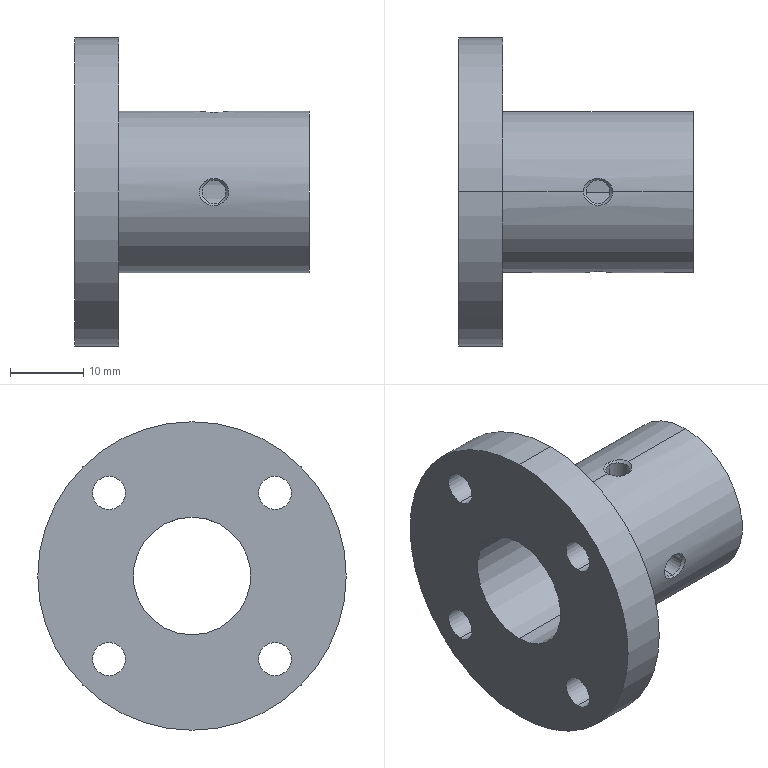Part | STEP file | STHRB16_STHRB16 | 1 solid | 35 faces | box 32 x 42 x 42 mm | volume 11327 mm3 | cylinder 24 | cone 8 | plane 3 | commonest cylinder face diameters 4.5 x8 4 x6 3.242 x4 16 x2 22 x2 42 x2
STEP:
#1=CARTESIAN_POINT('',(19.,-1.621,10.621));
#2=VERTEX_POINT('',#1);
#3=CARTESIAN_POINT('',(19.,1.621,10.621));
#4=VERTEX_POINT('',#3);
#5=CARTESIAN_POINT('',(19.,0.,10.621));
#6=DIRECTION('',(0.,0.,-1.));
#7=DIRECTION('',(0.,1.,0.));
#8=AXIS2_PLACEMENT_3D('',#5,#6,#7);
#9=CIRCLE('',#8,1.621);
#10=EDGE_CURVE('',#2,#4,#9,.T.);
#11=ORIENTED_EDGE('',*,*,#10,.F.);
#12=CARTESIAN_POINT('',(19.,-1.621,8.379));
#13=VERTEX_POINT('',#12);
#14=CARTESIAN_POINT('',(19.,-1.621,11.));
#15=DIRECTION('',(0.,0.,-1.));
#16=VECTOR('',#15,1000.);
#17=LINE('',#14,#16);
#18=EDGE_CURVE('',#2,#13,#17,.T.);
#19=ORIENTED_EDGE('',*,*,#18,.T.);
#20=CARTESIAN_POINT('',(19.,1.621,8.379));
#21=VERTEX_POINT('',#20);
#22=CARTESIAN_POINT('',(19.,0.,8.379));
#23=DIRECTION('',(0.,0.,-1.));
#24=DIRECTION('',(0.,1.,0.));
#25=AXIS2_PLACEMENT_3D('',#22,#23,#24);
#26=CIRCLE('',#25,1.621);
#27=EDGE_CURVE('',#13,#21,#26,.T.);
#28=ORIENTED_EDGE('',*,*,#27,.T.);
#29=CARTESIAN_POINT('',(19.,1.621,11.));
#30=DIRECTION('',(0.,0.,-1.));
#31=VECTOR('',#30,1000.);
#32=LINE('',#29,#31);
#33=EDGE_CURVE('',#4,#21,#32,.T.);
#34=ORIENTED_EDGE('',*,*,#33,.F.);
#35=EDGE_LOOP('',(#11,#19,#28,#34));
#36=FACE_OUTER_BOUND('',#35,.T.);
#37=CARTESIAN_POINT('',(19.,0.,11.));
#38=DIRECTION('',(0.,0.,-1.));
#39=DIRECTION('',(0.,1.,0.));
#40=AXIS2_PLACEMENT_3D('',#37,#38,#39);
#41=CYLINDRICAL_SURFACE('',#40,1.621);
#42=ADVANCED_FACE('',(#36),#41,.F.);
#43=ORIENTED_EDGE('',*,*,#27,.F.);
#44=CARTESIAN_POINT('',(19.,-2.,8.));
#45=VERTEX_POINT('',#44);
#46=CARTESIAN_POINT('',(19.,-1.621,8.379));
#47=DIRECTION('',(0.,-0.7071,-0.7071));
#48=VECTOR('',#47,1000.);
#49=LINE('',#46,#48);
#50=EDGE_CURVE('',#13,#45,#49,.T.);
#51=ORIENTED_EDGE('',*,*,#50,.T.);
#52=CARTESIAN_POINT('',(17.,0.,8.));
#53=VERTEX_POINT('',#52);
#54=CARTESIAN_POINT('',(19.,0.,8.));
#55=DIRECTION('',(0.,0.,-1.));
#56=DIRECTION('',(0.,1.,0.));
#57=AXIS2_PLACEMENT_3D('',#54,#55,#56);
#58=CIRCLE('',#57,2.);
#59=EDGE_CURVE('',#45,#53,#58,.T.);
#60=ORIENTED_EDGE('',*,*,#59,.T.);
#61=CARTESIAN_POINT('',(19.,2.,8.));
#62=VERTEX_POINT('',#61);
#63=CARTESIAN_POINT('',(19.,0.,8.));
#64=DIRECTION('',(0.,0.,-1.));
#65=DIRECTION('',(0.,1.,0.));
#66=AXIS2_PLACEMENT_3D('',#63,#64,#65);
#67=CIRCLE('',#66,2.);
#68=EDGE_CURVE('',#53,#62,#67,.T.);
#69=ORIENTED_EDGE('',*,*,#68,.T.);
#70=CARTESIAN_POINT('',(19.,1.621,8.379));
#71=DIRECTION('',(0.,0.7071,-0.7071));
#72=VECTOR('',#71,1000.);
#73=LINE('',#70,#72);
#74=EDGE_CURVE('',#21,#62,#73,.T.);
#75=ORIENTED_EDGE('',*,*,#74,.F.);
#76=EDGE_LOOP('',(#43,#51,#60,#69,#75));
#77=FACE_OUTER_BOUND('',#76,.T.);
#78=CARTESIAN_POINT('',(19.,0.,8.379));
#79=DIRECTION('',(0.,0.,-1.));
#80=DIRECTION('',(0.,1.,0.));
#81=AXIS2_PLACEMENT_3D('',#78,#79,#80);
#82=CONICAL_SURFACE('',#81,1.621,0.7854);
#83=ADVANCED_FACE('',(#77),#82,.F.);
#84=ORIENTED_EDGE('',*,*,#10,.T.);
#85=CARTESIAN_POINT('',(19.,1.844,10.844));
#86=VERTEX_POINT('',#85);
#87=CARTESIAN_POINT('',(19.,2.,11.));
#88=DIRECTION('',(0.,0.7071,0.7071));
#89=VECTOR('',#88,1000.);
#90=LINE('',#87,#89);
#91=EDGE_CURVE('',#4,#86,#90,.T.);
#92=ORIENTED_EDGE('',*,*,#91,.T.);
#93=CARTESIAN_POINT('',(17.,0.,11.));
#94=VERTEX_POINT('',#93);
#95=CARTESIAN_POINT('',(19.,1.844,10.844));
#96=CARTESIAN_POINT('',(18.874,1.844,10.844));
#97=CARTESIAN_POINT('',(18.747,1.833,10.846));
#98=CARTESIAN_POINT('',(18.499,1.789,10.854));
#99=CARTESIAN_POINT('',(18.378,1.756,10.859));
#100=CARTESIAN_POINT('',(18.142,1.669,10.873));
#101=CARTESIAN_POINT('',(18.027,1.615,10.881));
#102=CARTESIAN_POINT('',(17.811,1.486,10.899));
#103=CARTESIAN_POINT('',(17.71,1.413,10.909));
#104=CARTESIAN_POINT('',(17.522,1.247,10.929));
#105=CARTESIAN_POINT('',(17.435,1.153,10.94));
#106=CARTESIAN_POINT('',(17.284,0.9535,10.959));
#107=CARTESIAN_POINT('',(17.219,0.8468,10.968));
#108=CARTESIAN_POINT('',(17.058,0.5039,10.991));
#109=CARTESIAN_POINT('',(17.,0.2536,11.));
#110=CARTESIAN_POINT('',(17.,0.,11.));
#111=B_SPLINE_CURVE_WITH_KNOTS('',3,(#95,#96,#97,#98,#99,#100,#101,#102,#103,#104,#105,#106,#107,#108,#109,#110),.UNSPECIFIED.,.F.,.F.,(4,2,2,2,2,2,2,4),(0.007522,0.0079,0.008277,0.008655,0.009033,0.009411,0.009788,0.01054),.UNSPECIFIED.);
#112=EDGE_CURVE('',#86,#94,#111,.T.);
#113=ORIENTED_EDGE('',*,*,#112,.T.);
#114=CARTESIAN_POINT('',(19.,-1.844,10.844));
#115=VERTEX_POINT('',#114);
#116=CARTESIAN_POINT('',(17.,0.,11.));
#117=CARTESIAN_POINT('',(17.,-0.1265,11.));
#118=CARTESIAN_POINT('',(17.014,-0.2511,10.998));
#119=CARTESIAN_POINT('',(17.069,-0.4966,10.989));
#120=CARTESIAN_POINT('',(17.111,-0.6176,10.983));
#121=CARTESIAN_POINT('',(17.271,-0.958,10.961));
#122=CARTESIAN_POINT('',(17.427,-1.163,10.94));
#123=CARTESIAN_POINT('',(17.711,-1.414,10.909));
#124=CARTESIAN_POINT('',(17.813,-1.488,10.899));
#125=CARTESIAN_POINT('',(18.029,-1.616,10.881));
#126=CARTESIAN_POINT('',(18.144,-1.67,10.873));
#127=CARTESIAN_POINT('',(18.379,-1.757,10.859));
#128=CARTESIAN_POINT('',(18.5,-1.789,10.854));
#129=CARTESIAN_POINT('',(18.748,-1.833,10.846));
#130=CARTESIAN_POINT('',(18.875,-1.844,10.844));
#131=CARTESIAN_POINT('',(19.,-1.844,10.844));
#132=B_SPLINE_CURVE_WITH_KNOTS('',3,(#116,#117,#118,#119,#120,#121,#122,#123,#124,#125,#126,#127,#128,#129,#130,#131),.UNSPECIFIED.,.F.,.F.,(4,2,2,2,2,2,2,4),(0.01054,0.01092,0.0113,0.01205,0.01243,0.01281,0.01318,0.01356),.UNSPECIFIED.);
#133=EDGE_CURVE('',#94,#115,#132,.T.);
#134=ORIENTED_EDGE('',*,*,#133,.T.);
#135=CARTESIAN_POINT('',(19.,-2.,11.));
#136=DIRECTION('',(0.,-0.7071,0.7071));
#137=VECTOR('',#136,1000.);
#138=LINE('',#135,#137);
#139=EDGE_CURVE('',#2,#115,#138,.T.);
#140=ORIENTED_EDGE('',*,*,#139,.F.);
#141=EDGE_LOOP('',(#84,#92,#113,#134,#140));
#142=FACE_OUTER_BOUND('',#141,.T.);
#143=CARTESIAN_POINT('',(19.,0.,11.));
#144=DIRECTION('',(0.,0.,1.));
#145=DIRECTION('',(0.,-1.,0.));
#146=AXIS2_PLACEMENT_3D('',#143,#144,#145);
#147=CONICAL_SURFACE('',#146,2.,0.7854);
#148=ADVANCED_FACE('',(#142),#147,.F.);
#149=CARTESIAN_POINT('',(21.,0.,8.));
#150=VERTEX_POINT('',#149);
#151=CARTESIAN_POINT('',(19.,0.,8.));
#152=DIRECTION('',(0.,0.,-1.));
#153=DIRECTION('',(0.,1.,0.));
#154=AXIS2_PLACEMENT_3D('',#151,#152,#153);
#155=CIRCLE('',#154,2.);
#156=EDGE_CURVE('',#62,#150,#155,.T.);
#157=ORIENTED_EDGE('',*,*,#156,.F.);
#158=CARTESIAN_POINT('',(19.,2.,7.746));
#159=VERTEX_POINT('',#158);
#160=CARTESIAN_POINT('',(19.,2.,11.));
#161=DIRECTION('',(0.,0.,-1.));
#162=VECTOR('',#161,1000.);
#163=LINE('',#160,#162);
#164=EDGE_CURVE('',#62,#159,#163,.T.);
#165=ORIENTED_EDGE('',*,*,#164,.T.);
#166=CARTESIAN_POINT('',(19.,2.,7.746));
#167=CARTESIAN_POINT('',(19.132,2.,7.746));
#168=CARTESIAN_POINT('',(19.262,1.987,7.749));
#169=CARTESIAN_POINT('',(19.519,1.936,7.762));
#170=CARTESIAN_POINT('',(19.646,1.897,7.772));
#171=CARTESIAN_POINT('',(20.008,1.747,7.808));
#172=CARTESIAN_POINT('',(20.23,1.598,7.841));
#173=CARTESIAN_POINT('',(20.597,1.231,7.907));
#174=CARTESIAN_POINT('',(20.746,1.009,7.94));
#175=CARTESIAN_POINT('',(20.896,0.6485,7.975));
#176=CARTESIAN_POINT('',(20.935,0.5211,7.984));
#177=CARTESIAN_POINT('',(20.987,0.2634,7.997));
#178=CARTESIAN_POINT('',(21.,0.1326,8.));
#179=CARTESIAN_POINT('',(21.,0.,8.));
#180=B_SPLINE_CURVE_WITH_KNOTS('',3,(#166,#167,#168,#169,#170,#171,#172,#173,#174,#175,#176,#177,#178,#179),.UNSPECIFIED.,.F.,.F.,(4,2,2,2,2,2,4),(0.009417,0.009809,0.0102,0.01099,0.01177,0.01216,0.01255),.UNSPECIFIED.);
#181=EDGE_CURVE('',#159,#150,#180,.T.);
#182=ORIENTED_EDGE('',*,*,#181,.T.);
#183=EDGE_LOOP('',(#157,#165,#182));
#184=FACE_OUTER_BOUND('',#183,.T.);
#185=CARTESIAN_POINT('',(19.,0.,11.));
#186=DIRECTION('',(0.,0.,-1.));
#187=DIRECTION('',(0.,1.,0.));
#188=AXIS2_PLACEMENT_3D('',#185,#186,#187);
#189=CYLINDRICAL_SURFACE('',#188,2.);
#190=ADVANCED_FACE('',(#184),#189,.F.);
#191=CARTESIAN_POINT('',(19.,-10.621,-1.621));
#192=VERTEX_POINT('',#191);
#193=CARTESIAN_POINT('',(19.,-10.621,1.621));
#194=VERTEX_POINT('',#193);
#195=CARTESIAN_POINT('',(19.,-10.621,0.));
#196=DIRECTION('',(0.,1.,0.));
#197=DIRECTION('',(0.,0.,1.));
#198=AXIS2_PLACEMENT_3D('',#195,#196,#197);
#199=CIRCLE('',#198,1.621);
#200=EDGE_CURVE('',#192,#194,#199,.T.);
#201=ORIENTED_EDGE('',*,*,#200,.F.);
#202=CARTESIAN_POINT('',(19.,-8.379,-1.621));
#203=VERTEX_POINT('',#202);
#204=CARTESIAN_POINT('',(19.,-11.,-1.621));
#205=DIRECTION('',(0.,1.,0.));
#206=VECTOR('',#205,1000.);
#207=LINE('',#204,#206);
#208=EDGE_CURVE('',#192,#203,#207,.T.);
#209=ORIENTED_EDGE('',*,*,#208,.T.);
#210=CARTESIAN_POINT('',(19.,-8.379,1.621));
#211=VERTEX_POINT('',#210);
#212=CARTESIAN_POINT('',(19.,-8.379,0.));
#213=DIRECTION('',(0.,1.,0.));
#214=DIRECTION('',(0.,0.,1.));
#215=AXIS2_PLACEMENT_3D('',#212,#213,#214);
#216=CIRCLE('',#215,1.621);
#217=EDGE_CURVE('',#203,#211,#216,.T.);
#218=ORIENTED_EDGE('',*,*,#217,.T.);
#219=CARTESIAN_POINT('',(19.,-11.,1.621));
#220=DIRECTION('',(0.,1.,0.));
#221=VECTOR('',#220,1000.);
#222=LINE('',#219,#221);
#223=EDGE_CURVE('',#194,#211,#222,.T.);
#224=ORIENTED_EDGE('',*,*,#223,.F.);
#225=EDGE_LOOP('',(#201,#209,#218,#224));
#226=FACE_OUTER_BOUND('',#225,.T.);
#227=CARTESIAN_POINT('',(19.,-11.,0.));
#228=DIRECTION('',(0.,1.,0.));
#229=DIRECTION('',(0.,0.,1.));
#230=AXIS2_PLACEMENT_3D('',#227,#228,#229);
#231=CYLINDRICAL_SURFACE('',#230,1.621);
#232=ADVANCED_FACE('',(#226),#231,.F.);
#233=ORIENTED_EDGE('',*,*,#217,.F.);
#234=CARTESIAN_POINT('',(19.,-8.,-2.));
#235=VERTEX_POINT('',#234);
#236=CARTESIAN_POINT('',(19.,-8.379,-1.621));
#237=DIRECTION('',(0.,0.7071,-0.7071));
#238=VECTOR('',#237,1000.);
#239=LINE('',#236,#238);
#240=EDGE_CURVE('',#203,#235,#239,.T.);
#241=ORIENTED_EDGE('',*,*,#240,.T.);
#242=CARTESIAN_POINT('',(17.,-8.,0.));
#243=VERTEX_POINT('',#242);
#244=CARTESIAN_POINT('',(19.,-8.,0.));
#245=DIRECTION('',(0.,1.,0.));
#246=DIRECTION('',(0.,0.,1.));
#247=AXIS2_PLACEMENT_3D('',#244,#245,#246);
#248=CIRCLE('',#247,2.);
#249=EDGE_CURVE('',#235,#243,#248,.T.);
#250=ORIENTED_EDGE('',*,*,#249,.T.);
#251=CARTESIAN_POINT('',(19.,-8.,2.));
#252=VERTEX_POINT('',#251);
#253=CARTESIAN_POINT('',(19.,-8.,0.));
#254=DIRECTION('',(0.,1.,0.));
#255=DIRECTION('',(0.,0.,1.));
#256=AXIS2_PLACEMENT_3D('',#253,#254,#255);
#257=CIRCLE('',#256,2.);
#258=EDGE_CURVE('',#243,#252,#257,.T.);
#259=ORIENTED_EDGE('',*,*,#258,.T.);
#260=CARTESIAN_POINT('',(19.,-8.379,1.621));
#261=DIRECTION('',(0.,0.7071,0.7071));
#262=VECTOR('',#261,1000.);
#263=LINE('',#260,#262);
#264=EDGE_CURVE('',#211,#252,#263,.T.);
#265=ORIENTED_EDGE('',*,*,#264,.F.);
#266=EDGE_LOOP('',(#233,#241,#250,#259,#265));
#267=FACE_OUTER_BOUND('',#266,.T.);
#268=CARTESIAN_POINT('',(19.,-8.379,0.));
#269=DIRECTION('',(0.,1.,0.));
#270=DIRECTION('',(0.,0.,1.));
#271=AXIS2_PLACEMENT_3D('',#268,#269,#270);
#272=CONICAL_SURFACE('',#271,1.621,0.7854);
#273=ADVANCED_FACE('',(#267),#272,.F.);
#274=ORIENTED_EDGE('',*,*,#200,.T.);
#275=CARTESIAN_POINT('',(19.,-10.844,1.844));
#276=VERTEX_POINT('',#275);
#277=CARTESIAN_POINT('',(19.,-11.,2.));
#278=DIRECTION('',(0.,-0.7071,0.7071));
#279=VECTOR('',#278,1000.);
#280=LINE('',#277,#279);
#281=EDGE_CURVE('',#194,#276,#280,.T.);
#282=ORIENTED_EDGE('',*,*,#281,.T.);
#283=CARTESIAN_POINT('',(19.,-10.844,-1.844));
#284=VERTEX_POINT('',#283);
#285=CARTESIAN_POINT('',(19.,-10.844,1.844));
#286=CARTESIAN_POINT('',(18.874,-10.844,1.844));
#287=CARTESIAN_POINT('',(18.747,-10.846,1.833));
#288=CARTESIAN_POINT('',(18.499,-10.854,1.789));
#289=CARTESIAN_POINT('',(18.379,-10.859,1.756));
#290=CARTESIAN_POINT('',(18.143,-10.873,1.67));
#291=CARTESIAN_POINT('',(18.028,-10.881,1.615));
#292=CARTESIAN_POINT('',(17.812,-10.899,1.487));
#293=CARTESIAN_POINT('',(17.711,-10.909,1.414));
#294=CARTESIAN_POINT('',(17.523,-10.929,1.248));
#295=CARTESIAN_POINT('',(17.436,-10.94,1.154));
#296=CARTESIAN_POINT('',(17.285,-10.959,0.9553));
#297=CARTESIAN_POINT('',(17.22,-10.968,0.8487));
#298=CARTESIAN_POINT('',(17.058,-10.991,0.5066));
#299=CARTESIAN_POINT('',(17.,-11.,0.2567));
#300=CARTESIAN_POINT('',(17.,-11.,-0.1234));
#301=CARTESIAN_POINT('',(17.014,-10.998,-0.2482));
#302=CARTESIAN_POINT('',(17.069,-10.99,-0.494));
#303=CARTESIAN_POINT('',(17.11,-10.983,-0.6152));
#304=CARTESIAN_POINT('',(17.27,-10.961,-0.9562));
#305=CARTESIAN_POINT('',(17.426,-10.94,-1.161));
#306=CARTESIAN_POINT('',(17.71,-10.909,-1.413));
#307=CARTESIAN_POINT('',(17.812,-10.899,-1.487));
#308=CARTESIAN_POINT('',(18.028,-10.881,-1.615));
#309=CARTESIAN_POINT('',(18.143,-10.873,-1.67));
#310=CARTESIAN_POINT('',(18.379,-10.859,-1.757));
#311=CARTESIAN_POINT('',(18.5,-10.854,-1.789));
#312=CARTESIAN_POINT('',(18.747,-10.846,-1.833));
#313=CARTESIAN_POINT('',(18.875,-10.844,-1.844));
#314=CARTESIAN_POINT('',(19.,-10.844,-1.844));
#315=B_SPLINE_CURVE_WITH_KNOTS('',3,(#285,#286,#287,#288,#289,#290,#291,#292,#293,#294,#295,#296,#297,#298,#299,#300,#301,#302,#303,#304,#305,#306,#307,#308,#309,#310,#311,#312,#313,#314),.UNSPECIFIED.,.F.,.F.,(4,2,2,2,2,2,2,2,2,2,2,2,2,2,4),(0.007522,0.007899,0.008277,0.008654,0.009031,0.009409,0.009786,0.01054,0.01092,0.0113,0.01205,0.01243,0.0128,0.01318,0.01356),.UNSPECIFIED.);
#316=EDGE_CURVE('',#276,#284,#315,.T.);
#317=ORIENTED_EDGE('',*,*,#316,.T.);
#318=CARTESIAN_POINT('',(19.,-11.,-2.));
#319=DIRECTION('',(0.,-0.7071,-0.7071));
#320=VECTOR('',#319,1000.);
#321=LINE('',#318,#320);
#322=EDGE_CURVE('',#192,#284,#321,.T.);
#323=ORIENTED_EDGE('',*,*,#322,.F.);
#324=EDGE_LOOP('',(#274,#282,#317,#323));
#325=FACE_OUTER_BOUND('',#324,.T.);
#326=CARTESIAN_POINT('',(19.,-11.,0.));
#327=DIRECTION('',(0.,-1.,0.));
#328=DIRECTION('',(0.,0.,-1.));
#329=AXIS2_PLACEMENT_3D('',#326,#327,#328);
#330=CONICAL_SURFACE('',#329,2.,0.7854);
#331=ADVANCED_FACE('',(#325),#330,.F.);
#332=CARTESIAN_POINT('',(21.,-8.,0.));
#333=VERTEX_POINT('',#332);
#334=CARTESIAN_POINT('',(19.,-8.,0.));
#335=DIRECTION('',(0.,1.,0.));
#336=DIRECTION('',(0.,0.,1.));
#337=AXIS2_PLACEMENT_3D('',#334,#335,#336);
#338=CIRCLE('',#337,2.);
#339=EDGE_CURVE('',#252,#333,#338,.T.);
#340=ORIENTED_EDGE('',*,*,#339,.F.);
#341=CARTESIAN_POINT('',(19.,-7.746,2.));
#342=VERTEX_POINT('',#341);
#343=CARTESIAN_POINT('',(19.,-11.,2.));
#344=DIRECTION('',(0.,1.,0.));
#345=VECTOR('',#344,1000.);
#346=LINE('',#343,#345);
#347=EDGE_CURVE('',#252,#342,#346,.T.);
#348=ORIENTED_EDGE('',*,*,#347,.T.);
#349=CARTESIAN_POINT('',(19.,-7.746,2.));
#350=CARTESIAN_POINT('',(19.131,-7.746,2.));
#351=CARTESIAN_POINT('',(19.264,-7.749,1.987));
#352=CARTESIAN_POINT('',(19.521,-7.762,1.935));
#353=CARTESIAN_POINT('',(19.646,-7.772,1.897));
#354=CARTESIAN_POINT('',(20.01,-7.808,1.746));
#355=CARTESIAN_POINT('',(20.23,-7.841,1.599));
#356=CARTESIAN_POINT('',(20.507,-7.891,1.321));
#357=CARTESIAN_POINT('',(20.59,-7.907,1.221));
#358=CARTESIAN_POINT('',(20.734,-7.937,1.004));
#359=CARTESIAN_POINT('',(20.797,-7.952,0.8872));
#360=CARTESIAN_POINT('',(20.897,-7.975,0.6458));
#361=CARTESIAN_POINT('',(20.935,-7.984,0.5211));
#362=CARTESIAN_POINT('',(20.987,-7.997,0.2636));
#363=CARTESIAN_POINT('',(21.,-8.,0.1308));
#364=CARTESIAN_POINT('',(21.,-8.,0.));
#365=B_SPLINE_CURVE_WITH_KNOTS('',3,(#349,#350,#351,#352,#353,#354,#355,#356,#357,#358,#359,#360,#361,#362,#363,#364),.UNSPECIFIED.,.F.,.F.,(4,2,2,2,2,2,2,4),(0.00314,0.003532,0.003924,0.004709,0.005101,0.005493,0.005886,0.006278),.UNSPECIFIED.);
#366=EDGE_CURVE('',#342,#333,#365,.T.);
#367=ORIENTED_EDGE('',*,*,#366,.T.);
#368=EDGE_LOOP('',(#340,#348,#367));
#369=FACE_OUTER_BOUND('',#368,.T.);
#370=CARTESIAN_POINT('',(19.,-11.,0.));
#371=DIRECTION('',(0.,1.,0.));
#372=DIRECTION('',(0.,0.,1.));
#373=AXIS2_PLACEMENT_3D('',#370,#371,#372);
#374=CYLINDRICAL_SURFACE('',#373,2.);
#375=ADVANCED_FACE('',(#369),#374,.F.);
#376=CARTESIAN_POINT('',(6.,-11.314,13.564));
#377=VERTEX_POINT('',#376);
#378=CARTESIAN_POINT('',(6.,-11.314,9.064));
#379=VERTEX_POINT('',#378);
#380=CARTESIAN_POINT('',(6.,-11.314,11.314));
#381=DIRECTION('',(1.,0.,0.));
#382=DIRECTION('',(0.,0.,-1.));
#383=AXIS2_PLACEMENT_3D('',#380,#381,#382);
#384=CIRCLE('',#383,2.25);
#385=EDGE_CURVE('',#377,#379,#384,.T.);
#386=ORIENTED_EDGE('',*,*,#385,.T.);
#387=CARTESIAN_POINT('',(0.,-11.314,9.064));
#388=VERTEX_POINT('',#387);
#389=CARTESIAN_POINT('',(6.,-11.314,9.064));
#390=DIRECTION('',(-1.,0.,0.));
#391=VECTOR('',#390,1000.);
#392=LINE('',#389,#391);
#393=EDGE_CURVE('',#379,#388,#392,.T.);
#394=ORIENTED_EDGE('',*,*,#393,.T.);
#395=CARTESIAN_POINT('',(0.,-11.314,13.564));
#396=VERTEX_POINT('',#395);
#397=CARTESIAN_POINT('',(0.,-11.314,11.314));
#398=DIRECTION('',(1.,0.,0.));
#399=DIRECTION('',(0.,0.,-1.));
#400=AXIS2_PLACEMENT_3D('',#397,#398,#399);
#401=CIRCLE('',#400,2.25);
#402=EDGE_CURVE('',#396,#388,#401,.T.);
#403=ORIENTED_EDGE('',*,*,#402,.F.);
#404=CARTESIAN_POINT('',(6.,-11.314,13.564));
#405=DIRECTION('',(-1.,0.,0.));
#406=VECTOR('',#405,1000.);
#407=LINE('',#404,#406);
#408=EDGE_CURVE('',#377,#396,#407,.T.);
#409=ORIENTED_EDGE('',*,*,#408,.F.);
#410=EDGE_LOOP('',(#386,#394,#403,#409));
#411=FACE_OUTER_BOUND('',#410,.T.);
#412=CARTESIAN_POINT('',(6.,-11.314,11.314));
#413=DIRECTION('',(-1.,0.,0.));
#414=DIRECTION('',(0.,0.,1.));
#415=AXIS2_PLACEMENT_3D('',#412,#413,#414);
#416=CYLINDRICAL_SURFACE('',#415,2.25);
#417=ADVANCED_FACE('',(#411),#416,.F.);
#418=CARTESIAN_POINT('',(6.,11.314,13.564));
#419=VERTEX_POINT('',#418);
#420=CARTESIAN_POINT('',(6.,11.314,9.064));
#421=VERTEX_POINT('',#420);
#422=CARTESIAN_POINT('',(6.,11.314,11.314));
#423=DIRECTION('',(1.,0.,0.));
#424=DIRECTION('',(0.,0.,-1.));
#425=AXIS2_PLACEMENT_3D('',#422,#423,#424);
#426=CIRCLE('',#425,2.25);
#427=EDGE_CURVE('',#419,#421,#426,.T.);
#428=ORIENTED_EDGE('',*,*,#427,.T.);
#429=CARTESIAN_POINT('',(0.,11.314,9.064));
#430=VERTEX_POINT('',#429);
#431=CARTESIAN_POINT('',(6.,11.314,9.064));
#432=DIRECTION('',(-1.,0.,0.));
#433=VECTOR('',#432,1000.);
#434=LINE('',#431,#433);
#435=EDGE_CURVE('',#421,#430,#434,.T.);
#436=ORIENTED_EDGE('',*,*,#435,.T.);
#437=CARTESIAN_POINT('',(0.,11.314,13.564));
#438=VERTEX_POINT('',#437);
#439=CARTESIAN_POINT('',(0.,11.314,11.314));
#440=DIRECTION('',(1.,0.,0.));
#441=DIRECTION('',(0.,0.,-1.));
#442=AXIS2_PLACEMENT_3D('',#439,#440,#441);
#443=CIRCLE('',#442,2.25);
#444=EDGE_CURVE('',#438,#430,#443,.T.);
#445=ORIENTED_EDGE('',*,*,#444,.F.);
#446=CARTESIAN_POINT('',(6.,11.314,13.564));
#447=DIRECTION('',(-1.,0.,0.));
#448=VECTOR('',#447,1000.);
#449=LINE('',#446,#448);
#450=EDGE_CURVE('',#419,#438,#449,.T.);
#451=ORIENTED_EDGE('',*,*,#450,.F.);
#452=EDGE_LOOP('',(#428,#436,#445,#451));
#453=FACE_OUTER_BOUND('',#452,.T.);
#454=CARTESIAN_POINT('',(6.,11.314,11.314));
#455=DIRECTION('',(-1.,0.,0.));
#456=DIRECTION('',(0.,0.,1.));
#457=AXIS2_PLACEMENT_3D('',#454,#455,#456);
#458=CYLINDRICAL_SURFACE('',#457,2.25);
#459=ADVANCED_FACE('',(#453),#458,.F.);
#460=CARTESIAN_POINT('',(6.,-11.314,-9.064));
#461=VERTEX_POINT('',#460);
#462=CARTESIAN_POINT('',(6.,-11.314,-13.564));
#463=VERTEX_POINT('',#462);
#464=CARTESIAN_POINT('',(6.,-11.314,-11.314));
#465=DIRECTION('',(1.,0.,0.));
#466=DIRECTION('',(0.,0.,-1.));
#467=AXIS2_PLACEMENT_3D('',#464,#465,#466);
#468=CIRCLE('',#467,2.25);
#469=EDGE_CURVE('',#461,#463,#468,.T.);
#470=ORIENTED_EDGE('',*,*,#469,.T.);
#471=CARTESIAN_POINT('',(0.,-11.314,-13.564));
#472=VERTEX_POINT('',#471);
#473=CARTESIAN_POINT('',(6.,-11.314,-13.564));
#474=DIRECTION('',(-1.,0.,0.));
#475=VECTOR('',#474,1000.);
#476=LINE('',#473,#475);
#477=EDGE_CURVE('',#463,#472,#476,.T.);
#478=ORIENTED_EDGE('',*,*,#477,.T.);
#479=CARTESIAN_POINT('',(0.,-11.314,-9.064));
#480=VERTEX_POINT('',#479);
#481=CARTESIAN_POINT('',(0.,-11.314,-11.314));
#482=DIRECTION('',(1.,0.,0.));
#483=DIRECTION('',(0.,0.,-1.));
#484=AXIS2_PLACEMENT_3D('',#481,#482,#483);
#485=CIRCLE('',#484,2.25);
#486=EDGE_CURVE('',#480,#472,#485,.T.);
#487=ORIENTED_EDGE('',*,*,#486,.F.);
#488=CARTESIAN_POINT('',(6.,-11.314,-9.064));
#489=DIRECTION('',(-1.,0.,0.));
#490=VECTOR('',#489,1000.);
#491=LINE('',#488,#490);
#492=EDGE_CURVE('',#461,#480,#491,.T.);
#493=ORIENTED_EDGE('',*,*,#492,.F.);
#494=EDGE_LOOP('',(#470,#478,#487,#493));
#495=FACE_OUTER_BOUND('',#494,.T.);
#496=CARTESIAN_POINT('',(6.,-11.314,-11.314));
#497=DIRECTION('',(-1.,0.,0.));
#498=DIRECTION('',(0.,0.,1.));
#499=AXIS2_PLACEMENT_3D('',#496,#497,#498);
#500=CYLINDRICAL_SURFACE('',#499,2.25);
#501=ADVANCED_FACE('',(#495),#500,.F.);
#502=CARTESIAN_POINT('',(6.,11.314,-9.064));
#503=VERTEX_POINT('',#502);
#504=CARTESIAN_POINT('',(6.,11.314,-13.564));
#505=VERTEX_POINT('',#504);
#506=CARTESIAN_POINT('',(6.,11.314,-11.314));
#507=DIRECTION('',(1.,0.,0.));
#508=DIRECTION('',(0.,0.,-1.));
#509=AXIS2_PLACEMENT_3D('',#506,#507,#508);
#510=CIRCLE('',#509,2.25);
#511=EDGE_CURVE('',#503,#505,#510,.T.);
#512=ORIENTED_EDGE('',*,*,#511,.T.);
#513=CARTESIAN_POINT('',(0.,11.314,-13.564));
#514=VERTEX_POINT('',#513);
#515=CARTESIAN_POINT('',(6.,11.314,-13.564));
#516=DIRECTION('',(-1.,0.,0.));
#517=VECTOR('',#516,1000.);
#518=LINE('',#515,#517);
#519=EDGE_CURVE('',#505,#514,#518,.T.);
#520=ORIENTED_EDGE('',*,*,#519,.T.);
#521=CARTESIAN_POINT('',(0.,11.314,-9.064));
#522=VERTEX_POINT('',#521);
#523=CARTESIAN_POINT('',(0.,11.314,-11.314));
#524=DIRECTION('',(1.,0.,0.));
#525=DIRECTION('',(0.,0.,-1.));
#526=AXIS2_PLACEMENT_3D('',#523,#524,#525);
#527=CIRCLE('',#526,2.25);
#528=EDGE_CURVE('',#522,#514,#527,.T.);
#529=ORIENTED_EDGE('',*,*,#528,.F.);
#530=CARTESIAN_POINT('',(6.,11.314,-9.064));
#531=DIRECTION('',(-1.,0.,0.));
#532=VECTOR('',#531,1000.);
#533=LINE('',#530,#532);
#534=EDGE_CURVE('',#503,#522,#533,.T.);
#535=ORIENTED_EDGE('',*,*,#534,.F.);
#536=EDGE_LOOP('',(#512,#520,#529,#535));
#537=FACE_OUTER_BOUND('',#536,.T.);
#538=CARTESIAN_POINT('',(6.,11.314,-11.314));
#539=DIRECTION('',(-1.,0.,0.));
#540=DIRECTION('',(0.,0.,1.));
#541=AXIS2_PLACEMENT_3D('',#538,#539,#540);
#542=CYLINDRICAL_SURFACE('',#541,2.25);
#543=ADVANCED_FACE('',(#537),#542,.F.);
#544=CARTESIAN_POINT('',(6.,0.,21.));
#545=VERTEX_POINT('',#544);
#546=CARTESIAN_POINT('',(6.,0.,-21.));
#547=VERTEX_POINT('',#546);
#548=CARTESIAN_POINT('',(6.,0.,0.));
#549=DIRECTION('',(-1.,0.,0.));
#550=DIRECTION('',(0.,0.,1.));
#551=AXIS2_PLACEMENT_3D('',#548,#549,#550);
#552=CIRCLE('',#551,21.);
#553=EDGE_CURVE('',#545,#547,#552,.T.);
#554=ORIENTED_EDGE('',*,*,#553,.T.);
#555=CARTESIAN_POINT('',(0.,0.,-21.));
#556=VERTEX_POINT('',#555);
#557=CARTESIAN_POINT('',(32.,0.,-21.));
#558=DIRECTION('',(-1.,0.,0.));
#559=VECTOR('',#558,1000.);
#560=LINE('',#557,#559);
#561=EDGE_CURVE('',#547,#556,#560,.T.);
#562=ORIENTED_EDGE('',*,*,#561,.T.);
#563=CARTESIAN_POINT('',(0.,0.,21.));
#564=VERTEX_POINT('',#563);
#565=CARTESIAN_POINT('',(0.,0.,0.));
#566=DIRECTION('',(-1.,0.,0.));
#567=DIRECTION('',(0.,0.,1.));
#568=AXIS2_PLACEMENT_3D('',#565,#566,#567);
#569=CIRCLE('',#568,21.);
#570=EDGE_CURVE('',#564,#556,#569,.T.);
#571=ORIENTED_EDGE('',*,*,#570,.F.);
#572=CARTESIAN_POINT('',(32.,0.,21.));
#573=DIRECTION('',(-1.,0.,0.));
#574=VECTOR('',#573,1000.);
#575=LINE('',#572,#574);
#576=EDGE_CURVE('',#545,#564,#575,.T.);
#577=ORIENTED_EDGE('',*,*,#576,.F.);
#578=EDGE_LOOP('',(#554,#562,#571,#577));
#579=FACE_OUTER_BOUND('',#578,.T.);
#580=CARTESIAN_POINT('',(32.,0.,0.));
#581=DIRECTION('',(-1.,0.,0.));
#582=DIRECTION('',(0.,0.,1.));
#583=AXIS2_PLACEMENT_3D('',#580,#581,#582);
#584=CYLINDRICAL_SURFACE('',#583,21.);
#585=ADVANCED_FACE('',(#579),#584,.T.);
#586=CARTESIAN_POINT('',(32.,0.,11.));
#587=VERTEX_POINT('',#586);
#588=CARTESIAN_POINT('',(32.,0.,-11.));
#589=VERTEX_POINT('',#588);
#590=CARTESIAN_POINT('',(32.,0.,0.));
#591=DIRECTION('',(-1.,0.,0.));
#592=DIRECTION('',(0.,0.,1.));
#593=AXIS2_PLACEMENT_3D('',#590,#591,#592);
#594=CIRCLE('',#593,11.);
#595=EDGE_CURVE('',#587,#589,#594,.T.);
#596=ORIENTED_EDGE('',*,*,#595,.T.);
#597=CARTESIAN_POINT('',(6.,0.,-11.));
#598=VERTEX_POINT('',#597);
#599=CARTESIAN_POINT('',(32.,0.,-11.));
#600=DIRECTION('',(-1.,0.,0.));
#601=VECTOR('',#600,1000.);
#602=LINE('',#599,#601);
#603=EDGE_CURVE('',#589,#598,#602,.T.);
#604=ORIENTED_EDGE('',*,*,#603,.T.);
#605=CARTESIAN_POINT('',(6.,0.,11.));
#606=VERTEX_POINT('',#605);
#607=CARTESIAN_POINT('',(6.,0.,0.));
#608=DIRECTION('',(-1.,0.,0.));
#609=DIRECTION('',(0.,0.,1.));
#610=AXIS2_PLACEMENT_3D('',#607,#608,#609);
#611=CIRCLE('',#610,11.);
#612=EDGE_CURVE('',#606,#598,#611,.T.);
#613=ORIENTED_EDGE('',*,*,#612,.F.);
#614=CARTESIAN_POINT('',(32.,0.,11.));
#615=DIRECTION('',(-1.,0.,0.));
#616=VECTOR('',#615,1000.);
#617=LINE('',#614,#616);
#618=EDGE_CURVE('',#94,#606,#617,.T.);
#619=ORIENTED_EDGE('',*,*,#618,.F.);
#620=ORIENTED_EDGE('',*,*,#112,.F.);
#621=CARTESIAN_POINT('',(21.,0.,11.));
#622=VERTEX_POINT('',#621);
#623=CARTESIAN_POINT('',(21.,0.,11.));
#624=CARTESIAN_POINT('',(21.,0.1258,11.));
#625=CARTESIAN_POINT('',(20.986,0.2533,10.998));
#626=CARTESIAN_POINT('',(20.93,0.498,10.989));
#627=CARTESIAN_POINT('',(20.889,0.6178,10.983));
#628=CARTESIAN_POINT('',(20.781,0.8466,10.968));
#629=CARTESIAN_POINT('',(20.716,0.9536,10.959));
#630=CARTESIAN_POINT('',(20.564,1.154,10.94));
#631=CARTESIAN_POINT('',(20.477,1.247,10.929));
#632=CARTESIAN_POINT('',(20.196,1.496,10.899));
#633=CARTESIAN_POINT('',(19.974,1.627,10.879));
#634=CARTESIAN_POINT('',(19.622,1.756,10.859));
#635=CARTESIAN_POINT('',(19.499,1.79,10.853));
#636=CARTESIAN_POINT('',(19.25,1.833,10.846));
#637=CARTESIAN_POINT('',(19.125,1.844,10.844));
#638=CARTESIAN_POINT('',(19.,1.844,10.844));
#639=B_SPLINE_CURVE_WITH_KNOTS('',3,(#623,#624,#625,#626,#627,#628,#629,#630,#631,#632,#633,#634,#635,#636,#637,#638),.UNSPECIFIED.,.F.,.F.,(4,2,2,2,2,2,2,4),(0.004504,0.004881,0.005259,0.005636,0.006013,0.006768,0.007145,0.007522),.UNSPECIFIED.);
#640=EDGE_CURVE('',#622,#86,#639,.T.);
#641=ORIENTED_EDGE('',*,*,#640,.F.);
#642=CARTESIAN_POINT('',(32.,0.,11.));
#643=DIRECTION('',(-1.,0.,0.));
#644=VECTOR('',#643,1000.);
#645=LINE('',#642,#644);
#646=EDGE_CURVE('',#587,#622,#645,.T.);
#647=ORIENTED_EDGE('',*,*,#646,.F.);
#648=EDGE_LOOP('',(#596,#604,#613,#619,#620,#641,#647));
#649=FACE_OUTER_BOUND('',#648,.T.);
#650=CARTESIAN_POINT('',(32.,0.,0.));
#651=DIRECTION('',(-1.,0.,0.));
#652=DIRECTION('',(0.,0.,1.));
#653=AXIS2_PLACEMENT_3D('',#650,#651,#652);
#654=CYLINDRICAL_SURFACE('',#653,11.);
#655=ADVANCED_FACE('',(#649),#654,.T.);
#656=CARTESIAN_POINT('',(17.,-8.,0.));
#657=CARTESIAN_POINT('',(17.,-8.,0.1327));
#658=CARTESIAN_POINT('',(17.013,-7.997,0.2632));
#659=CARTESIAN_POINT('',(17.064,-7.984,0.5196));
#660=CARTESIAN_POINT('',(17.103,-7.975,0.647));
#661=CARTESIAN_POINT('',(17.204,-7.951,0.889));
#662=CARTESIAN_POINT('',(17.265,-7.938,1.004));
#663=CARTESIAN_POINT('',(17.41,-7.907,1.221));
#664=CARTESIAN_POINT('',(17.495,-7.89,1.323));
#665=CARTESIAN_POINT('',(17.77,-7.841,1.599));
#666=CARTESIAN_POINT('',(17.993,-7.808,1.747));
#667=CARTESIAN_POINT('',(18.354,-7.772,1.897));
#668=CARTESIAN_POINT('',(18.48,-7.762,1.936));
#669=CARTESIAN_POINT('',(18.739,-7.749,1.987));
#670=CARTESIAN_POINT('',(18.869,-7.746,2.));
#671=CARTESIAN_POINT('',(19.,-7.746,2.));
#672=B_SPLINE_CURVE_WITH_KNOTS('',3,(#656,#657,#658,#659,#660,#661,#662,#663,#664,#665,#666,#667,#668,#669,#670,#671),.UNSPECIFIED.,.F.,.F.,(4,2,2,2,2,2,2,4),(0.,0.0003925,0.0007849,0.001177,0.00157,0.002355,0.002747,0.00314),.UNSPECIFIED.);
#673=EDGE_CURVE('',#243,#342,#672,.T.);
#674=ORIENTED_EDGE('',*,*,#673,.F.);
#675=CARTESIAN_POINT('',(21.,-8.,0.));
#676=CARTESIAN_POINT('',(21.,-8.,-0.2616));
#677=CARTESIAN_POINT('',(20.947,-7.986,-0.5257));
#678=CARTESIAN_POINT('',(20.797,-7.952,-0.8871));
#679=CARTESIAN_POINT('',(20.735,-7.937,-1.004));
#680=CARTESIAN_POINT('',(20.589,-7.907,-1.221));
#681=CARTESIAN_POINT('',(20.507,-7.891,-1.321));
#682=CARTESIAN_POINT('',(20.323,-7.858,-1.506));
#683=CARTESIAN_POINT('',(20.22,-7.841,-1.59));
#684=CARTESIAN_POINT('',(20.004,-7.81,-1.734));
#685=CARTESIAN_POINT('',(19.89,-7.796,-1.796));
#686=CARTESIAN_POINT('',(19.525,-7.76,-1.948));
#687=CARTESIAN_POINT('',(19.264,-7.746,-2.));
#688=CARTESIAN_POINT('',(18.869,-7.746,-2.));
#689=CARTESIAN_POINT('',(18.739,-7.749,-1.987));
#690=CARTESIAN_POINT('',(18.482,-7.762,-1.936));
#691=CARTESIAN_POINT('',(18.354,-7.772,-1.897));
#692=CARTESIAN_POINT('',(17.992,-7.808,-1.747));
#693=CARTESIAN_POINT('',(17.77,-7.841,-1.598));
#694=CARTESIAN_POINT('',(17.403,-7.907,-1.232));
#695=CARTESIAN_POINT('',(17.254,-7.94,-1.01));
#696=CARTESIAN_POINT('',(17.104,-7.975,-0.6486));
#697=CARTESIAN_POINT('',(17.065,-7.984,-0.5212));
#698=CARTESIAN_POINT('',(17.013,-7.997,-0.2634));
#699=CARTESIAN_POINT('',(17.,-8.,-0.1327));
#700=CARTESIAN_POINT('',(17.,-8.,0.));
#701=B_SPLINE_CURVE_WITH_KNOTS('',3,(#675,#676,#677,#678,#679,#680,#681,#682,#683,#684,#685,#686,#687,#688,#689,#690,#691,#692,#693,#694,#695,#696,#697,#698,#699,#700),.UNSPECIFIED.,.F.,.F.,(4,2,2,2,2,2,2,2,2,2,2,2,4),(0.006278,0.007062,0.007455,0.007847,0.008239,0.008631,0.009416,0.009808,0.0102,0.01099,0.01177,0.01216,0.01255),.UNSPECIFIED.);
#702=EDGE_CURVE('',#333,#243,#701,.T.);
#703=ORIENTED_EDGE('',*,*,#702,.F.);
#704=ORIENTED_EDGE('',*,*,#366,.F.);
#705=EDGE_LOOP('',(#674,#703,#704));
#706=FACE_BOUND('',#705,.T.);
#707=CARTESIAN_POINT('',(32.,0.,-8.));
#708=VERTEX_POINT('',#707);
#709=CARTESIAN_POINT('',(32.,0.,8.));
#710=VERTEX_POINT('',#709);
#711=CARTESIAN_POINT('',(32.,0.,0.));
#712=DIRECTION('',(-1.,0.,0.));
#713=DIRECTION('',(0.,0.,1.));
#714=AXIS2_PLACEMENT_3D('',#711,#712,#713);
#715=CIRCLE('',#714,8.);
#716=EDGE_CURVE('',#708,#710,#715,.T.);
#717=ORIENTED_EDGE('',*,*,#716,.F.);
#718=CARTESIAN_POINT('',(0.,0.,-8.));
#719=VERTEX_POINT('',#718);
#720=CARTESIAN_POINT('',(32.,0.,-8.));
#721=DIRECTION('',(-1.,0.,0.));
#722=VECTOR('',#721,1000.);
#723=LINE('',#720,#722);
#724=EDGE_CURVE('',#708,#719,#723,.T.);
#725=ORIENTED_EDGE('',*,*,#724,.T.);
#726=CARTESIAN_POINT('',(0.,0.,8.));
#727=VERTEX_POINT('',#726);
#728=CARTESIAN_POINT('',(0.,0.,0.));
#729=DIRECTION('',(-1.,0.,0.));
#730=DIRECTION('',(0.,0.,1.));
#731=AXIS2_PLACEMENT_3D('',#728,#729,#730);
#732=CIRCLE('',#731,8.);
#733=EDGE_CURVE('',#719,#727,#732,.T.);
#734=ORIENTED_EDGE('',*,*,#733,.T.);
#735=CARTESIAN_POINT('',(32.,0.,8.));
#736=DIRECTION('',(-1.,0.,0.));
#737=VECTOR('',#736,1000.);
#738=LINE('',#735,#737);
#739=EDGE_CURVE('',#53,#727,#738,.T.);
#740=ORIENTED_EDGE('',*,*,#739,.F.);
#741=CARTESIAN_POINT('',(21.,0.,8.));
#742=CARTESIAN_POINT('',(21.,-0.1327,8.));
#743=CARTESIAN_POINT('',(20.987,-0.2631,7.997));
#744=CARTESIAN_POINT('',(20.936,-0.5195,7.984));
#745=CARTESIAN_POINT('',(20.897,-0.6468,7.975));
#746=CARTESIAN_POINT('',(20.796,-0.8888,7.951));
#747=CARTESIAN_POINT('',(20.735,-1.003,7.938));
#748=CARTESIAN_POINT('',(20.59,-1.22,7.907));
#749=CARTESIAN_POINT('',(20.506,-1.323,7.89));
#750=CARTESIAN_POINT('',(20.23,-1.598,7.841));
#751=CARTESIAN_POINT('',(20.008,-1.747,7.808));
#752=CARTESIAN_POINT('',(19.647,-1.897,7.772));
#753=CARTESIAN_POINT('',(19.52,-1.936,7.762));
#754=CARTESIAN_POINT('',(19.262,-1.987,7.749));
#755=CARTESIAN_POINT('',(19.132,-2.,7.746));
#756=CARTESIAN_POINT('',(18.87,-2.,7.746));
#757=CARTESIAN_POINT('',(18.737,-1.987,7.749));
#758=CARTESIAN_POINT('',(18.48,-1.936,7.762));
#759=CARTESIAN_POINT('',(18.355,-1.898,7.772));
#760=CARTESIAN_POINT('',(17.991,-1.746,7.808));
#761=CARTESIAN_POINT('',(17.771,-1.599,7.841));
#762=CARTESIAN_POINT('',(17.493,-1.321,7.891));
#763=CARTESIAN_POINT('',(17.41,-1.221,7.907));
#764=CARTESIAN_POINT('',(17.266,-1.005,7.937));
#765=CARTESIAN_POINT('',(17.203,-0.8874,7.952));
#766=CARTESIAN_POINT('',(17.103,-0.646,7.975));
#767=CARTESIAN_POINT('',(17.065,-0.5212,7.984));
#768=CARTESIAN_POINT('',(17.013,-0.2636,7.997));
#769=CARTESIAN_POINT('',(17.,-0.1308,8.));
#770=CARTESIAN_POINT('',(17.,0.,8.));
#771=B_SPLINE_CURVE_WITH_KNOTS('',3,(#741,#742,#743,#744,#745,#746,#747,#748,#749,#750,#751,#752,#753,#754,#755,#756,#757,#758,#759,#760,#761,#762,#763,#764,#765,#766,#767,#768,#769,#770),.UNSPECIFIED.,.F.,.F.,(4,2,2,2,2,2,2,2,2,2,2,2,2,2,4),(0.,0.0003924,0.0007847,0.001177,0.001569,0.002354,0.002747,0.003139,0.003531,0.003924,0.004708,0.005101,0.005493,0.005886,0.006278),.UNSPECIFIED.);
#772=EDGE_CURVE('',#150,#53,#771,.T.);
#773=ORIENTED_EDGE('',*,*,#772,.F.);
#774=CARTESIAN_POINT('',(32.,0.,8.));
#775=DIRECTION('',(-1.,0.,0.));
#776=VECTOR('',#775,1000.);
#777=LINE('',#774,#776);
#778=EDGE_CURVE('',#710,#150,#777,.T.);
#779=ORIENTED_EDGE('',*,*,#778,.F.);
#780=EDGE_LOOP('',(#717,#725,#734,#740,#773,#779));
#781=FACE_OUTER_BOUND('',#780,.T.);
#782=CARTESIAN_POINT('',(32.,0.,0.));
#783=DIRECTION('',(-1.,0.,0.));
#784=DIRECTION('',(0.,0.,1.));
#785=AXIS2_PLACEMENT_3D('',#782,#783,#784);
#786=CYLINDRICAL_SURFACE('',#785,8.);
#787=ADVANCED_FACE('',(#706,#781),#786,.F.);
#788=ORIENTED_EDGE('',*,*,#724,.F.);
#789=CARTESIAN_POINT('',(32.,0.,0.));
#790=DIRECTION('',(-1.,0.,0.));
#791=DIRECTION('',(0.,0.,1.));
#792=AXIS2_PLACEMENT_3D('',#789,#790,#791);
#793=CIRCLE('',#792,8.);
#794=EDGE_CURVE('',#710,#708,#793,.T.);
#795=ORIENTED_EDGE('',*,*,#794,.F.);
#796=ORIENTED_EDGE('',*,*,#778,.T.);
#797=ORIENTED_EDGE('',*,*,#181,.F.);
#798=CARTESIAN_POINT('',(17.,0.,8.));
#799=CARTESIAN_POINT('',(17.,0.2617,8.));
#800=CARTESIAN_POINT('',(17.053,0.5258,7.986));
#801=CARTESIAN_POINT('',(17.203,0.8872,7.952));
#802=CARTESIAN_POINT('',(17.265,1.004,7.937));
#803=CARTESIAN_POINT('',(17.411,1.221,7.907));
#804=CARTESIAN_POINT('',(17.493,1.322,7.891));
#805=CARTESIAN_POINT('',(17.678,1.506,7.858));
#806=CARTESIAN_POINT('',(17.78,1.59,7.841));
#807=CARTESIAN_POINT('',(17.996,1.735,7.81));
#808=CARTESIAN_POINT('',(18.111,1.796,7.796));
#809=CARTESIAN_POINT('',(18.476,1.948,7.76));
#810=CARTESIAN_POINT('',(18.736,2.,7.746));
#811=CARTESIAN_POINT('',(19.,2.,7.746));
#812=B_SPLINE_CURVE_WITH_KNOTS('',3,(#798,#799,#800,#801,#802,#803,#804,#805,#806,#807,#808,#809,#810,#811),.UNSPECIFIED.,.F.,.F.,(4,2,2,2,2,2,4),(0.006278,0.007063,0.007455,0.007847,0.00824,0.008632,0.009417),.UNSPECIFIED.);
#813=EDGE_CURVE('',#53,#159,#812,.T.);
#814=ORIENTED_EDGE('',*,*,#813,.F.);
#815=ORIENTED_EDGE('',*,*,#739,.T.);
#816=CARTESIAN_POINT('',(0.,0.,0.));
#817=DIRECTION('',(-1.,0.,0.));
#818=DIRECTION('',(0.,0.,1.));
#819=AXIS2_PLACEMENT_3D('',#816,#817,#818);
#820=CIRCLE('',#819,8.);
#821=EDGE_CURVE('',#727,#719,#820,.T.);
#822=ORIENTED_EDGE('',*,*,#821,.T.);
#823=EDGE_LOOP('',(#788,#795,#796,#797,#814,#815,#822));
#824=FACE_OUTER_BOUND('',#823,.T.);
#825=CARTESIAN_POINT('',(32.,0.,0.));
#826=DIRECTION('',(-1.,0.,0.));
#827=DIRECTION('',(0.,0.,1.));
#828=AXIS2_PLACEMENT_3D('',#825,#826,#827);
#829=CYLINDRICAL_SURFACE('',#828,8.);
#830=ADVANCED_FACE('',(#824),#829,.F.);
#831=ORIENTED_EDGE('',*,*,#603,.F.);
#832=CARTESIAN_POINT('',(32.,0.,0.));
#833=DIRECTION('',(-1.,0.,0.));
#834=DIRECTION('',(0.,0.,1.));
#835=AXIS2_PLACEMENT_3D('',#832,#833,#834);
#836=CIRCLE('',#835,11.);
#837=EDGE_CURVE('',#589,#587,#836,.T.);
#838=ORIENTED_EDGE('',*,*,#837,.T.);
#839=ORIENTED_EDGE('',*,*,#646,.T.);
#840=CARTESIAN_POINT('',(19.,-1.844,10.844));
#841=CARTESIAN_POINT('',(19.126,-1.844,10.844));
#842=CARTESIAN_POINT('',(19.251,-1.833,10.846));
#843=CARTESIAN_POINT('',(19.5,-1.789,10.854));
#844=CARTESIAN_POINT('',(19.623,-1.756,10.859));
#845=CARTESIAN_POINT('',(19.976,-1.626,10.88));
#846=CARTESIAN_POINT('',(20.198,-1.495,10.899));
#847=CARTESIAN_POINT('',(20.572,-1.164,10.94));
#848=CARTESIAN_POINT('',(20.729,-0.9581,10.961));
#849=CARTESIAN_POINT('',(20.888,-0.6184,10.983));
#850=CARTESIAN_POINT('',(20.93,-0.4977,10.989));
#851=CARTESIAN_POINT('',(20.986,-0.2509,10.998));
#852=CARTESIAN_POINT('',(21.,-0.1262,11.));
#853=CARTESIAN_POINT('',(21.,0.,11.));
#854=B_SPLINE_CURVE_WITH_KNOTS('',3,(#840,#841,#842,#843,#844,#845,#846,#847,#848,#849,#850,#851,#852,#853),.UNSPECIFIED.,.F.,.F.,(4,2,2,2,2,2,4),(0.001479,0.001857,0.002235,0.002991,0.003748,0.004126,0.004504),.UNSPECIFIED.);
#855=EDGE_CURVE('',#115,#622,#854,.T.);
#856=ORIENTED_EDGE('',*,*,#855,.F.);
#857=ORIENTED_EDGE('',*,*,#133,.F.);
#858=ORIENTED_EDGE('',*,*,#618,.T.);
#859=CARTESIAN_POINT('',(6.,0.,0.));
#860=DIRECTION('',(-1.,0.,0.));
#861=DIRECTION('',(0.,0.,1.));
#862=AXIS2_PLACEMENT_3D('',#859,#860,#861);
#863=CIRCLE('',#862,11.);
#864=EDGE_CURVE('',#598,#606,#863,.T.);
#865=ORIENTED_EDGE('',*,*,#864,.F.);
#866=EDGE_LOOP('',(#831,#838,#839,#856,#857,#858,#865));
#867=FACE_OUTER_BOUND('',#866,.T.);
#868=CARTESIAN_POINT('',(19.,-10.844,-1.844));
#869=CARTESIAN_POINT('',(19.126,-10.844,-1.844));
#870=CARTESIAN_POINT('',(19.25,-10.846,-1.833));
#871=CARTESIAN_POINT('',(19.499,-10.853,-1.79));
#872=CARTESIAN_POINT('',(19.622,-10.859,-1.756));
#873=CARTESIAN_POINT('',(19.974,-10.879,-1.626));
#874=CARTESIAN_POINT('',(20.196,-10.899,-1.496));
#875=CARTESIAN_POINT('',(20.57,-10.939,-1.165));
#876=CARTESIAN_POINT('',(20.727,-10.96,-0.9603));
#877=CARTESIAN_POINT('',(20.887,-10.983,-0.6213));
#878=CARTESIAN_POINT('',(20.929,-10.989,-0.5009));
#879=CARTESIAN_POINT('',(20.985,-10.998,-0.2545));
#880=CARTESIAN_POINT('',(21.,-11.,-0.1299));
#881=CARTESIAN_POINT('',(21.,-11.,0.122));
#882=CARTESIAN_POINT('',(20.986,-10.998,0.2497));
#883=CARTESIAN_POINT('',(20.931,-10.99,0.4949));
#884=CARTESIAN_POINT('',(20.89,-10.983,0.6149));
#885=CARTESIAN_POINT('',(20.782,-10.968,0.8442));
#886=CARTESIAN_POINT('',(20.717,-10.959,0.9515));
#887=CARTESIAN_POINT('',(20.566,-10.94,1.152));
#888=CARTESIAN_POINT('',(20.479,-10.93,1.246));
#889=CARTESIAN_POINT('',(20.197,-10.899,1.495));
#890=CARTESIAN_POINT('',(19.976,-10.88,1.626));
#891=CARTESIAN_POINT('',(19.622,-10.859,1.756));
#892=CARTESIAN_POINT('',(19.5,-10.854,1.789));
#893=CARTESIAN_POINT('',(19.251,-10.846,1.833));
#894=CARTESIAN_POINT('',(19.126,-10.844,1.844));
#895=CARTESIAN_POINT('',(19.,-10.844,1.844));
#896=B_SPLINE_CURVE_WITH_KNOTS('',3,(#868,#869,#870,#871,#872,#873,#874,#875,#876,#877,#878,#879,#880,#881,#882,#883,#884,#885,#886,#887,#888,#889,#890,#891,#892,#893,#894,#895),.UNSPECIFIED.,.F.,.F.,(4,2,2,2,2,2,2,2,2,2,2,2,2,4),(0.001479,0.001856,0.002234,0.00299,0.003745,0.004123,0.0045,0.004878,0.005256,0.005633,0.006011,0.006767,0.007144,0.007522),.UNSPECIFIED.);
#897=EDGE_CURVE('',#284,#276,#896,.T.);
#898=ORIENTED_EDGE('',*,*,#897,.F.);
#899=ORIENTED_EDGE('',*,*,#316,.F.);
#900=EDGE_LOOP('',(#898,#899));
#901=FACE_BOUND('',#900,.T.);
#902=CARTESIAN_POINT('',(32.,0.,0.));
#903=DIRECTION('',(-1.,0.,0.));
#904=DIRECTION('',(0.,0.,1.));
#905=AXIS2_PLACEMENT_3D('',#902,#903,#904);
#906=CYLINDRICAL_SURFACE('',#905,11.);
#907=ADVANCED_FACE('',(#867,#901),#906,.T.);
#908=ORIENTED_EDGE('',*,*,#444,.T.);
#909=CARTESIAN_POINT('',(0.,11.314,11.314));
#910=DIRECTION('',(1.,0.,0.));
#911=DIRECTION('',(0.,0.,-1.));
#912=AXIS2_PLACEMENT_3D('',#909,#910,#911);
#913=CIRCLE('',#912,2.25);
#914=EDGE_CURVE('',#430,#438,#913,.T.);
#915=ORIENTED_EDGE('',*,*,#914,.T.);
#916=EDGE_LOOP('',(#908,#915));
#917=FACE_BOUND('',#916,.T.);
#918=ORIENTED_EDGE('',*,*,#528,.T.);
#919=CARTESIAN_POINT('',(0.,11.314,-11.314));
#920=DIRECTION('',(1.,0.,0.));
#921=DIRECTION('',(0.,0.,-1.));
#922=AXIS2_PLACEMENT_3D('',#919,#920,#921);
#923=CIRCLE('',#922,2.25);
#924=EDGE_CURVE('',#514,#522,#923,.T.);
#925=ORIENTED_EDGE('',*,*,#924,.T.);
#926=EDGE_LOOP('',(#918,#925));
#927=FACE_BOUND('',#926,.T.);
#928=ORIENTED_EDGE('',*,*,#821,.F.);
#929=ORIENTED_EDGE('',*,*,#733,.F.);
#930=EDGE_LOOP('',(#928,#929));
#931=FACE_BOUND('',#930,.T.);
#932=ORIENTED_EDGE('',*,*,#570,.T.);
#933=CARTESIAN_POINT('',(0.,0.,0.));
#934=DIRECTION('',(-1.,0.,0.));
#935=DIRECTION('',(0.,0.,1.));
#936=AXIS2_PLACEMENT_3D('',#933,#934,#935);
#937=CIRCLE('',#936,21.);
#938=EDGE_CURVE('',#556,#564,#937,.T.);
#939=ORIENTED_EDGE('',*,*,#938,.T.);
#940=EDGE_LOOP('',(#932,#939));
#941=FACE_OUTER_BOUND('',#940,.T.);
#942=ORIENTED_EDGE('',*,*,#486,.T.);
#943=CARTESIAN_POINT('',(0.,-11.314,-11.314));
#944=DIRECTION('',(1.,0.,0.));
#945=DIRECTION('',(0.,0.,-1.));
#946=AXIS2_PLACEMENT_3D('',#943,#944,#945);
#947=CIRCLE('',#946,2.25);
#948=EDGE_CURVE('',#472,#480,#947,.T.);
#949=ORIENTED_EDGE('',*,*,#948,.T.);
#950=EDGE_LOOP('',(#942,#949));
#951=FACE_BOUND('',#950,.T.);
#952=ORIENTED_EDGE('',*,*,#402,.T.);
#953=CARTESIAN_POINT('',(0.,-11.314,11.314));
#954=DIRECTION('',(1.,0.,0.));
#955=DIRECTION('',(0.,0.,-1.));
#956=AXIS2_PLACEMENT_3D('',#953,#954,#955);
#957=CIRCLE('',#956,2.25);
#958=EDGE_CURVE('',#388,#396,#957,.T.);
#959=ORIENTED_EDGE('',*,*,#958,.T.);
#960=EDGE_LOOP('',(#952,#959));
#961=FACE_BOUND('',#960,.T.);
#962=CARTESIAN_POINT('',(0.,21.,0.));
#963=DIRECTION('',(1.,0.,0.));
#964=DIRECTION('',(0.,0.,-1.));
#965=AXIS2_PLACEMENT_3D('',#962,#963,#964);
#966=PLANE('',#965);
#967=ADVANCED_FACE('',(#917,#927,#931,#941,#951,#961),#966,.F.);
#968=ORIENTED_EDGE('',*,*,#427,.F.);
#969=CARTESIAN_POINT('',(6.,11.314,11.314));
#970=DIRECTION('',(1.,0.,0.));
#971=DIRECTION('',(0.,0.,-1.));
#972=AXIS2_PLACEMENT_3D('',#969,#970,#971);
#973=CIRCLE('',#972,2.25);
#974=EDGE_CURVE('',#421,#419,#973,.T.);
#975=ORIENTED_EDGE('',*,*,#974,.F.);
#976=EDGE_LOOP('',(#968,#975));
#977=FACE_BOUND('',#976,.T.);
#978=ORIENTED_EDGE('',*,*,#511,.F.);
#979=CARTESIAN_POINT('',(6.,11.314,-11.314));
#980=DIRECTION('',(1.,0.,0.));
#981=DIRECTION('',(0.,0.,-1.));
#982=AXIS2_PLACEMENT_3D('',#979,#980,#981);
#983=CIRCLE('',#982,2.25);
#984=EDGE_CURVE('',#505,#503,#983,.T.);
#985=ORIENTED_EDGE('',*,*,#984,.F.);
#986=EDGE_LOOP('',(#978,#985));
#987=FACE_BOUND('',#986,.T.);
#988=ORIENTED_EDGE('',*,*,#553,.F.);
#989=CARTESIAN_POINT('',(6.,0.,0.));
#990=DIRECTION('',(-1.,0.,0.));
#991=DIRECTION('',(0.,0.,1.));
#992=AXIS2_PLACEMENT_3D('',#989,#990,#991);
#993=CIRCLE('',#992,21.);
#994=EDGE_CURVE('',#547,#545,#993,.T.);
#995=ORIENTED_EDGE('',*,*,#994,.F.);
#996=EDGE_LOOP('',(#988,#995));
#997=FACE_OUTER_BOUND('',#996,.T.);
#998=ORIENTED_EDGE('',*,*,#612,.T.);
#999=ORIENTED_EDGE('',*,*,#864,.T.);
#1000=EDGE_LOOP('',(#998,#999));
#1001=FACE_BOUND('',#1000,.T.);
#1002=ORIENTED_EDGE('',*,*,#469,.F.);
#1003=CARTESIAN_POINT('',(6.,-11.314,-11.314));
#1004=DIRECTION('',(1.,0.,0.));
#1005=DIRECTION('',(0.,0.,-1.));
#1006=AXIS2_PLACEMENT_3D('',#1003,#1004,#1005);
#1007=CIRCLE('',#1006,2.25);
#1008=EDGE_CURVE('',#463,#461,#1007,.T.);
#1009=ORIENTED_EDGE('',*,*,#1008,.F.);
#1010=EDGE_LOOP('',(#1002,#1009));
#1011=FACE_BOUND('',#1010,.T.);
#1012=ORIENTED_EDGE('',*,*,#385,.F.);
#1013=CARTESIAN_POINT('',(6.,-11.314,11.314));
#1014=DIRECTION('',(1.,0.,0.));
#1015=DIRECTION('',(0.,0.,-1.));
#1016=AXIS2_PLACEMENT_3D('',#1013,#1014,#1015);
#1017=CIRCLE('',#1016,2.25);
#1018=EDGE_CURVE('',#379,#377,#1017,.T.);
#1019=ORIENTED_EDGE('',*,*,#1018,.F.);
#1020=EDGE_LOOP('',(#1012,#1019));
#1021=FACE_BOUND('',#1020,.T.);
#1022=CARTESIAN_POINT('',(6.,11.,0.));
#1023=DIRECTION('',(-1.,0.,0.));
#1024=DIRECTION('',(0.,0.,1.));
#1025=AXIS2_PLACEMENT_3D('',#1022,#1023,#1024);
#1026=PLANE('',#1025);
#1027=ADVANCED_FACE('',(#977,#987,#997,#1001,#1011,#1021),#1026,.F.);
#1028=ORIENTED_EDGE('',*,*,#561,.F.);
#1029=ORIENTED_EDGE('',*,*,#994,.T.);
#1030=ORIENTED_EDGE('',*,*,#576,.T.);
#1031=ORIENTED_EDGE('',*,*,#938,.F.);
#1032=EDGE_LOOP('',(#1028,#1029,#1030,#1031));
#1033=FACE_OUTER_BOUND('',#1032,.T.);
#1034=CARTESIAN_POINT('',(32.,0.,0.));
#1035=DIRECTION('',(-1.,0.,0.));
#1036=DIRECTION('',(0.,0.,1.));
#1037=AXIS2_PLACEMENT_3D('',#1034,#1035,#1036);
#1038=CYLINDRICAL_SURFACE('',#1037,21.);
#1039=ADVANCED_FACE('',(#1033),#1038,.T.);
#1040=ORIENTED_EDGE('',*,*,#595,.F.);
#1041=ORIENTED_EDGE('',*,*,#837,.F.);
#1042=EDGE_LOOP('',(#1040,#1041));
#1043=FACE_OUTER_BOUND('',#1042,.T.);
#1044=ORIENTED_EDGE('',*,*,#794,.T.);
#1045=ORIENTED_EDGE('',*,*,#716,.T.);
#1046=EDGE_LOOP('',(#1044,#1045));
#1047=FACE_BOUND('',#1046,.T.);
#1048=CARTESIAN_POINT('',(32.,8.,0.));
#1049=DIRECTION('',(-1.,0.,0.));
#1050=DIRECTION('',(0.,0.,1.));
#1051=AXIS2_PLACEMENT_3D('',#1048,#1049,#1050);
#1052=PLANE('',#1051);
#1053=ADVANCED_FACE('',(#1043,#1047),#1052,.F.);
#1054=ORIENTED_EDGE('',*,*,#519,.F.);
#1055=ORIENTED_EDGE('',*,*,#984,.T.);
#1056=ORIENTED_EDGE('',*,*,#534,.T.);
#1057=ORIENTED_EDGE('',*,*,#924,.F.);
#1058=EDGE_LOOP('',(#1054,#1055,#1056,#1057));
#1059=FACE_OUTER_BOUND('',#1058,.T.);
#1060=CARTESIAN_POINT('',(6.,11.314,-11.314));
#1061=DIRECTION('',(-1.,0.,0.));
#1062=DIRECTION('',(0.,0.,1.));
#1063=AXIS2_PLACEMENT_3D('',#1060,#1061,#1062);
#1064=CYLINDRICAL_SURFACE('',#1063,2.25);
#1065=ADVANCED_FACE('',(#1059),#1064,.F.);
#1066=ORIENTED_EDGE('',*,*,#477,.F.);
#1067=ORIENTED_EDGE('',*,*,#1008,.T.);
#1068=ORIENTED_EDGE('',*,*,#492,.T.);
#1069=ORIENTED_EDGE('',*,*,#948,.F.);
#1070=EDGE_LOOP('',(#1066,#1067,#1068,#1069));
#1071=FACE_OUTER_BOUND('',#1070,.T.);
#1072=CARTESIAN_POINT('',(6.,-11.314,-11.314));
#1073=DIRECTION('',(-1.,0.,0.));
#1074=DIRECTION('',(0.,0.,1.));
#1075=AXIS2_PLACEMENT_3D('',#1072,#1073,#1074);
#1076=CYLINDRICAL_SURFACE('',#1075,2.25);
#1077=ADVANCED_FACE('',(#1071),#1076,.F.);
#1078=ORIENTED_EDGE('',*,*,#435,.F.);
#1079=ORIENTED_EDGE('',*,*,#974,.T.);
#1080=ORIENTED_EDGE('',*,*,#450,.T.);
#1081=ORIENTED_EDGE('',*,*,#914,.F.);
#1082=EDGE_LOOP('',(#1078,#1079,#1080,#1081));
#1083=FACE_OUTER_BOUND('',#1082,.T.);
#1084=CARTESIAN_POINT('',(6.,11.314,11.314));
#1085=DIRECTION('',(-1.,0.,0.));
#1086=DIRECTION('',(0.,0.,1.));
#1087=AXIS2_PLACEMENT_3D('',#1084,#1085,#1086);
#1088=CYLINDRICAL_SURFACE('',#1087,2.25);
#1089=ADVANCED_FACE('',(#1083),#1088,.F.);
#1090=ORIENTED_EDGE('',*,*,#393,.F.);
#1091=ORIENTED_EDGE('',*,*,#1018,.T.);
#1092=ORIENTED_EDGE('',*,*,#408,.T.);
#1093=ORIENTED_EDGE('',*,*,#958,.F.);
#1094=EDGE_LOOP('',(#1090,#1091,#1092,#1093));
#1095=FACE_OUTER_BOUND('',#1094,.T.);
#1096=CARTESIAN_POINT('',(6.,-11.314,11.314));
#1097=DIRECTION('',(-1.,0.,0.));
#1098=DIRECTION('',(0.,0.,1.));
#1099=AXIS2_PLACEMENT_3D('',#1096,#1097,#1098);
#1100=CYLINDRICAL_SURFACE('',#1099,2.25);
#1101=ADVANCED_FACE('',(#1095),#1100,.F.);
#1102=ORIENTED_EDGE('',*,*,#347,.F.);
#1103=ORIENTED_EDGE('',*,*,#258,.F.);
#1104=ORIENTED_EDGE('',*,*,#673,.T.);
#1105=EDGE_LOOP('',(#1102,#1103,#1104));
#1106=FACE_OUTER_BOUND('',#1105,.T.);
#1107=CARTESIAN_POINT('',(19.,-11.,0.));
#1108=DIRECTION('',(0.,1.,0.));
#1109=DIRECTION('',(0.,0.,1.));
#1110=AXIS2_PLACEMENT_3D('',#1107,#1108,#1109);
#1111=CYLINDRICAL_SURFACE('',#1110,2.);
#1112=ADVANCED_FACE('',(#1106),#1111,.F.);
#1113=ORIENTED_EDGE('',*,*,#702,.T.);
#1114=ORIENTED_EDGE('',*,*,#249,.F.);
#1115=CARTESIAN_POINT('',(19.,-8.,0.));
#1116=DIRECTION('',(0.,1.,0.));
#1117=DIRECTION('',(0.,0.,1.));
#1118=AXIS2_PLACEMENT_3D('',#1115,#1116,#1117);
#1119=CIRCLE('',#1118,2.);
#1120=EDGE_CURVE('',#333,#235,#1119,.T.);
#1121=ORIENTED_EDGE('',*,*,#1120,.F.);
#1122=EDGE_LOOP('',(#1113,#1114,#1121));
#1123=FACE_OUTER_BOUND('',#1122,.T.);
#1124=CARTESIAN_POINT('',(19.,-11.,0.));
#1125=DIRECTION('',(0.,1.,0.));
#1126=DIRECTION('',(0.,0.,1.));
#1127=AXIS2_PLACEMENT_3D('',#1124,#1125,#1126);
#1128=CYLINDRICAL_SURFACE('',#1127,2.);
#1129=ADVANCED_FACE('',(#1123),#1128,.F.);
#1130=ORIENTED_EDGE('',*,*,#281,.F.);
#1131=CARTESIAN_POINT('',(19.,-10.621,0.));
#1132=DIRECTION('',(0.,1.,0.));
#1133=DIRECTION('',(0.,0.,1.));
#1134=AXIS2_PLACEMENT_3D('',#1131,#1132,#1133);
#1135=CIRCLE('',#1134,1.621);
#1136=EDGE_CURVE('',#194,#192,#1135,.T.);
#1137=ORIENTED_EDGE('',*,*,#1136,.T.);
#1138=ORIENTED_EDGE('',*,*,#322,.T.);
#1139=ORIENTED_EDGE('',*,*,#897,.T.);
#1140=EDGE_LOOP('',(#1130,#1137,#1138,#1139));
#1141=FACE_OUTER_BOUND('',#1140,.T.);
#1142=CARTESIAN_POINT('',(19.,-11.,0.));
#1143=DIRECTION('',(0.,-1.,0.));
#1144=DIRECTION('',(0.,0.,-1.));
#1145=AXIS2_PLACEMENT_3D('',#1142,#1143,#1144);
#1146=CONICAL_SURFACE('',#1145,2.,0.7854);
#1147=ADVANCED_FACE('',(#1141),#1146,.F.);
#1148=ORIENTED_EDGE('',*,*,#240,.F.);
#1149=CARTESIAN_POINT('',(19.,-8.379,0.));
#1150=DIRECTION('',(0.,1.,0.));
#1151=DIRECTION('',(0.,0.,1.));
#1152=AXIS2_PLACEMENT_3D('',#1149,#1150,#1151);
#1153=CIRCLE('',#1152,1.621);
#1154=EDGE_CURVE('',#211,#203,#1153,.T.);
#1155=ORIENTED_EDGE('',*,*,#1154,.F.);
#1156=ORIENTED_EDGE('',*,*,#264,.T.);
#1157=ORIENTED_EDGE('',*,*,#339,.T.);
#1158=ORIENTED_EDGE('',*,*,#1120,.T.);
#1159=EDGE_LOOP('',(#1148,#1155,#1156,#1157,#1158));
#1160=FACE_OUTER_BOUND('',#1159,.T.);
#1161=CARTESIAN_POINT('',(19.,-8.379,0.));
#1162=DIRECTION('',(0.,1.,0.));
#1163=DIRECTION('',(0.,0.,1.));
#1164=AXIS2_PLACEMENT_3D('',#1161,#1162,#1163);
#1165=CONICAL_SURFACE('',#1164,1.621,0.7854);
#1166=ADVANCED_FACE('',(#1160),#1165,.F.);
#1167=ORIENTED_EDGE('',*,*,#208,.F.);
#1168=ORIENTED_EDGE('',*,*,#1136,.F.);
#1169=ORIENTED_EDGE('',*,*,#223,.T.);
#1170=ORIENTED_EDGE('',*,*,#1154,.T.);
#1171=EDGE_LOOP('',(#1167,#1168,#1169,#1170));
#1172=FACE_OUTER_BOUND('',#1171,.T.);
#1173=CARTESIAN_POINT('',(19.,-11.,0.));
#1174=DIRECTION('',(0.,1.,0.));
#1175=DIRECTION('',(0.,0.,1.));
#1176=AXIS2_PLACEMENT_3D('',#1173,#1174,#1175);
#1177=CYLINDRICAL_SURFACE('',#1176,1.621);
#1178=ADVANCED_FACE('',(#1172),#1177,.F.);
#1179=ORIENTED_EDGE('',*,*,#772,.T.);
#1180=ORIENTED_EDGE('',*,*,#59,.F.);
#1181=CARTESIAN_POINT('',(19.,0.,8.));
#1182=DIRECTION('',(0.,0.,-1.));
#1183=DIRECTION('',(0.,1.,0.));
#1184=AXIS2_PLACEMENT_3D('',#1181,#1182,#1183);
#1185=CIRCLE('',#1184,2.);
#1186=EDGE_CURVE('',#150,#45,#1185,.T.);
#1187=ORIENTED_EDGE('',*,*,#1186,.F.);
#1188=EDGE_LOOP('',(#1179,#1180,#1187));
#1189=FACE_OUTER_BOUND('',#1188,.T.);
#1190=CARTESIAN_POINT('',(19.,0.,11.));
#1191=DIRECTION('',(0.,0.,-1.));
#1192=DIRECTION('',(0.,1.,0.));
#1193=AXIS2_PLACEMENT_3D('',#1190,#1191,#1192);
#1194=CYLINDRICAL_SURFACE('',#1193,2.);
#1195=ADVANCED_FACE('',(#1189),#1194,.F.);
#1196=ORIENTED_EDGE('',*,*,#164,.F.);
#1197=ORIENTED_EDGE('',*,*,#68,.F.);
#1198=ORIENTED_EDGE('',*,*,#813,.T.);
#1199=EDGE_LOOP('',(#1196,#1197,#1198));
#1200=FACE_OUTER_BOUND('',#1199,.T.);
#1201=CARTESIAN_POINT('',(19.,0.,11.));
#1202=DIRECTION('',(0.,0.,-1.));
#1203=DIRECTION('',(0.,1.,0.));
#1204=AXIS2_PLACEMENT_3D('',#1201,#1202,#1203);
#1205=CYLINDRICAL_SURFACE('',#1204,2.);
#1206=ADVANCED_FACE('',(#1200),#1205,.F.);
#1207=ORIENTED_EDGE('',*,*,#91,.F.);
#1208=CARTESIAN_POINT('',(19.,0.,10.621));
#1209=DIRECTION('',(0.,0.,-1.));
#1210=DIRECTION('',(0.,1.,0.));
#1211=AXIS2_PLACEMENT_3D('',#1208,#1209,#1210);
#1212=CIRCLE('',#1211,1.621);
#1213=EDGE_CURVE('',#4,#2,#1212,.T.);
#1214=ORIENTED_EDGE('',*,*,#1213,.T.);
#1215=ORIENTED_EDGE('',*,*,#139,.T.);
#1216=ORIENTED_EDGE('',*,*,#855,.T.);
#1217=ORIENTED_EDGE('',*,*,#640,.T.);
#1218=EDGE_LOOP('',(#1207,#1214,#1215,#1216,#1217));
#1219=FACE_OUTER_BOUND('',#1218,.T.);
#1220=CARTESIAN_POINT('',(19.,0.,11.));
#1221=DIRECTION('',(0.,0.,1.));
#1222=DIRECTION('',(0.,-1.,0.));
#1223=AXIS2_PLACEMENT_3D('',#1220,#1221,#1222);
#1224=CONICAL_SURFACE('',#1223,2.,0.7854);
#1225=ADVANCED_FACE('',(#1219),#1224,.F.);
#1226=ORIENTED_EDGE('',*,*,#50,.F.);
#1227=CARTESIAN_POINT('',(19.,0.,8.379));
#1228=DIRECTION('',(0.,0.,-1.));
#1229=DIRECTION('',(0.,1.,0.));
#1230=AXIS2_PLACEMENT_3D('',#1227,#1228,#1229);
#1231=CIRCLE('',#1230,1.621);
#1232=EDGE_CURVE('',#21,#13,#1231,.T.);
#1233=ORIENTED_EDGE('',*,*,#1232,.F.);
#1234=ORIENTED_EDGE('',*,*,#74,.T.);
#1235=ORIENTED_EDGE('',*,*,#156,.T.);
#1236=ORIENTED_EDGE('',*,*,#1186,.T.);
#1237=EDGE_LOOP('',(#1226,#1233,#1234,#1235,#1236));
#1238=FACE_OUTER_BOUND('',#1237,.T.);
#1239=CARTESIAN_POINT('',(19.,0.,8.379));
#1240=DIRECTION('',(0.,0.,-1.));
#1241=DIRECTION('',(0.,1.,0.));
#1242=AXIS2_PLACEMENT_3D('',#1239,#1240,#1241);
#1243=CONICAL_SURFACE('',#1242,1.621,0.7854);
#1244=ADVANCED_FACE('',(#1238),#1243,.F.);
#1245=ORIENTED_EDGE('',*,*,#18,.F.);
#1246=ORIENTED_EDGE('',*,*,#1213,.F.);
#1247=ORIENTED_EDGE('',*,*,#33,.T.);
#1248=ORIENTED_EDGE('',*,*,#1232,.T.);
#1249=EDGE_LOOP('',(#1245,#1246,#1247,#1248));
#1250=FACE_OUTER_BOUND('',#1249,.T.);
#1251=CARTESIAN_POINT('',(19.,0.,11.));
#1252=DIRECTION('',(0.,0.,-1.));
#1253=DIRECTION('',(0.,1.,0.));
#1254=AXIS2_PLACEMENT_3D('',#1251,#1252,#1253);
#1255=CYLINDRICAL_SURFACE('',#1254,1.621);
#1256=ADVANCED_FACE('',(#1250),#1255,.F.);
#1257=CLOSED_SHELL('',(#42,#83,#148,#190,#232,#273,#331,#375,#417,#459,#501,#543,#585,#655,#787,#830,#907,#967,#1027,#1039,#1053,#1065,#1077,#1089,#1101,#1112,#1129,#1147,#1166,#1178,#1195,#1206,#1225,#1244,#1256));
#1258=MANIFOLD_SOLID_BREP('',#1257);
#1259=CARTESIAN_POINT('',(0.,0.,0.));
#1260=DIRECTION('',(0.,0.,1.));
#1261=DIRECTION('',(1.,0.,0.));
#1262=AXIS2_PLACEMENT_3D('',#1259,#1260,#1261);
#1263=(LENGTH_UNIT()NAMED_UNIT(*)SI_UNIT(.MILLI.,.METRE.));
#1264=UNCERTAINTY_MEASURE_WITH_UNIT(LENGTH_MEASURE(0.00001),#1263,'','');
#1265=(NAMED_UNIT(*)PLANE_ANGLE_UNIT()SI_UNIT($,.RADIAN.));
#1266=(NAMED_UNIT(*)SI_UNIT($,.STERADIAN.)SOLID_ANGLE_UNIT());
#1267=(GEOMETRIC_REPRESENTATION_CONTEXT(3)GLOBAL_UNCERTAINTY_ASSIGNED_CONTEXT((#1264))GLOBAL_UNIT_ASSIGNED_CONTEXT((#1263,#1265,#1266))REPRESENTATION_CONTEXT('',''));
#1268=ADVANCED_BREP_SHAPE_REPRESENTATION('',(#1258,#1262),#1267);